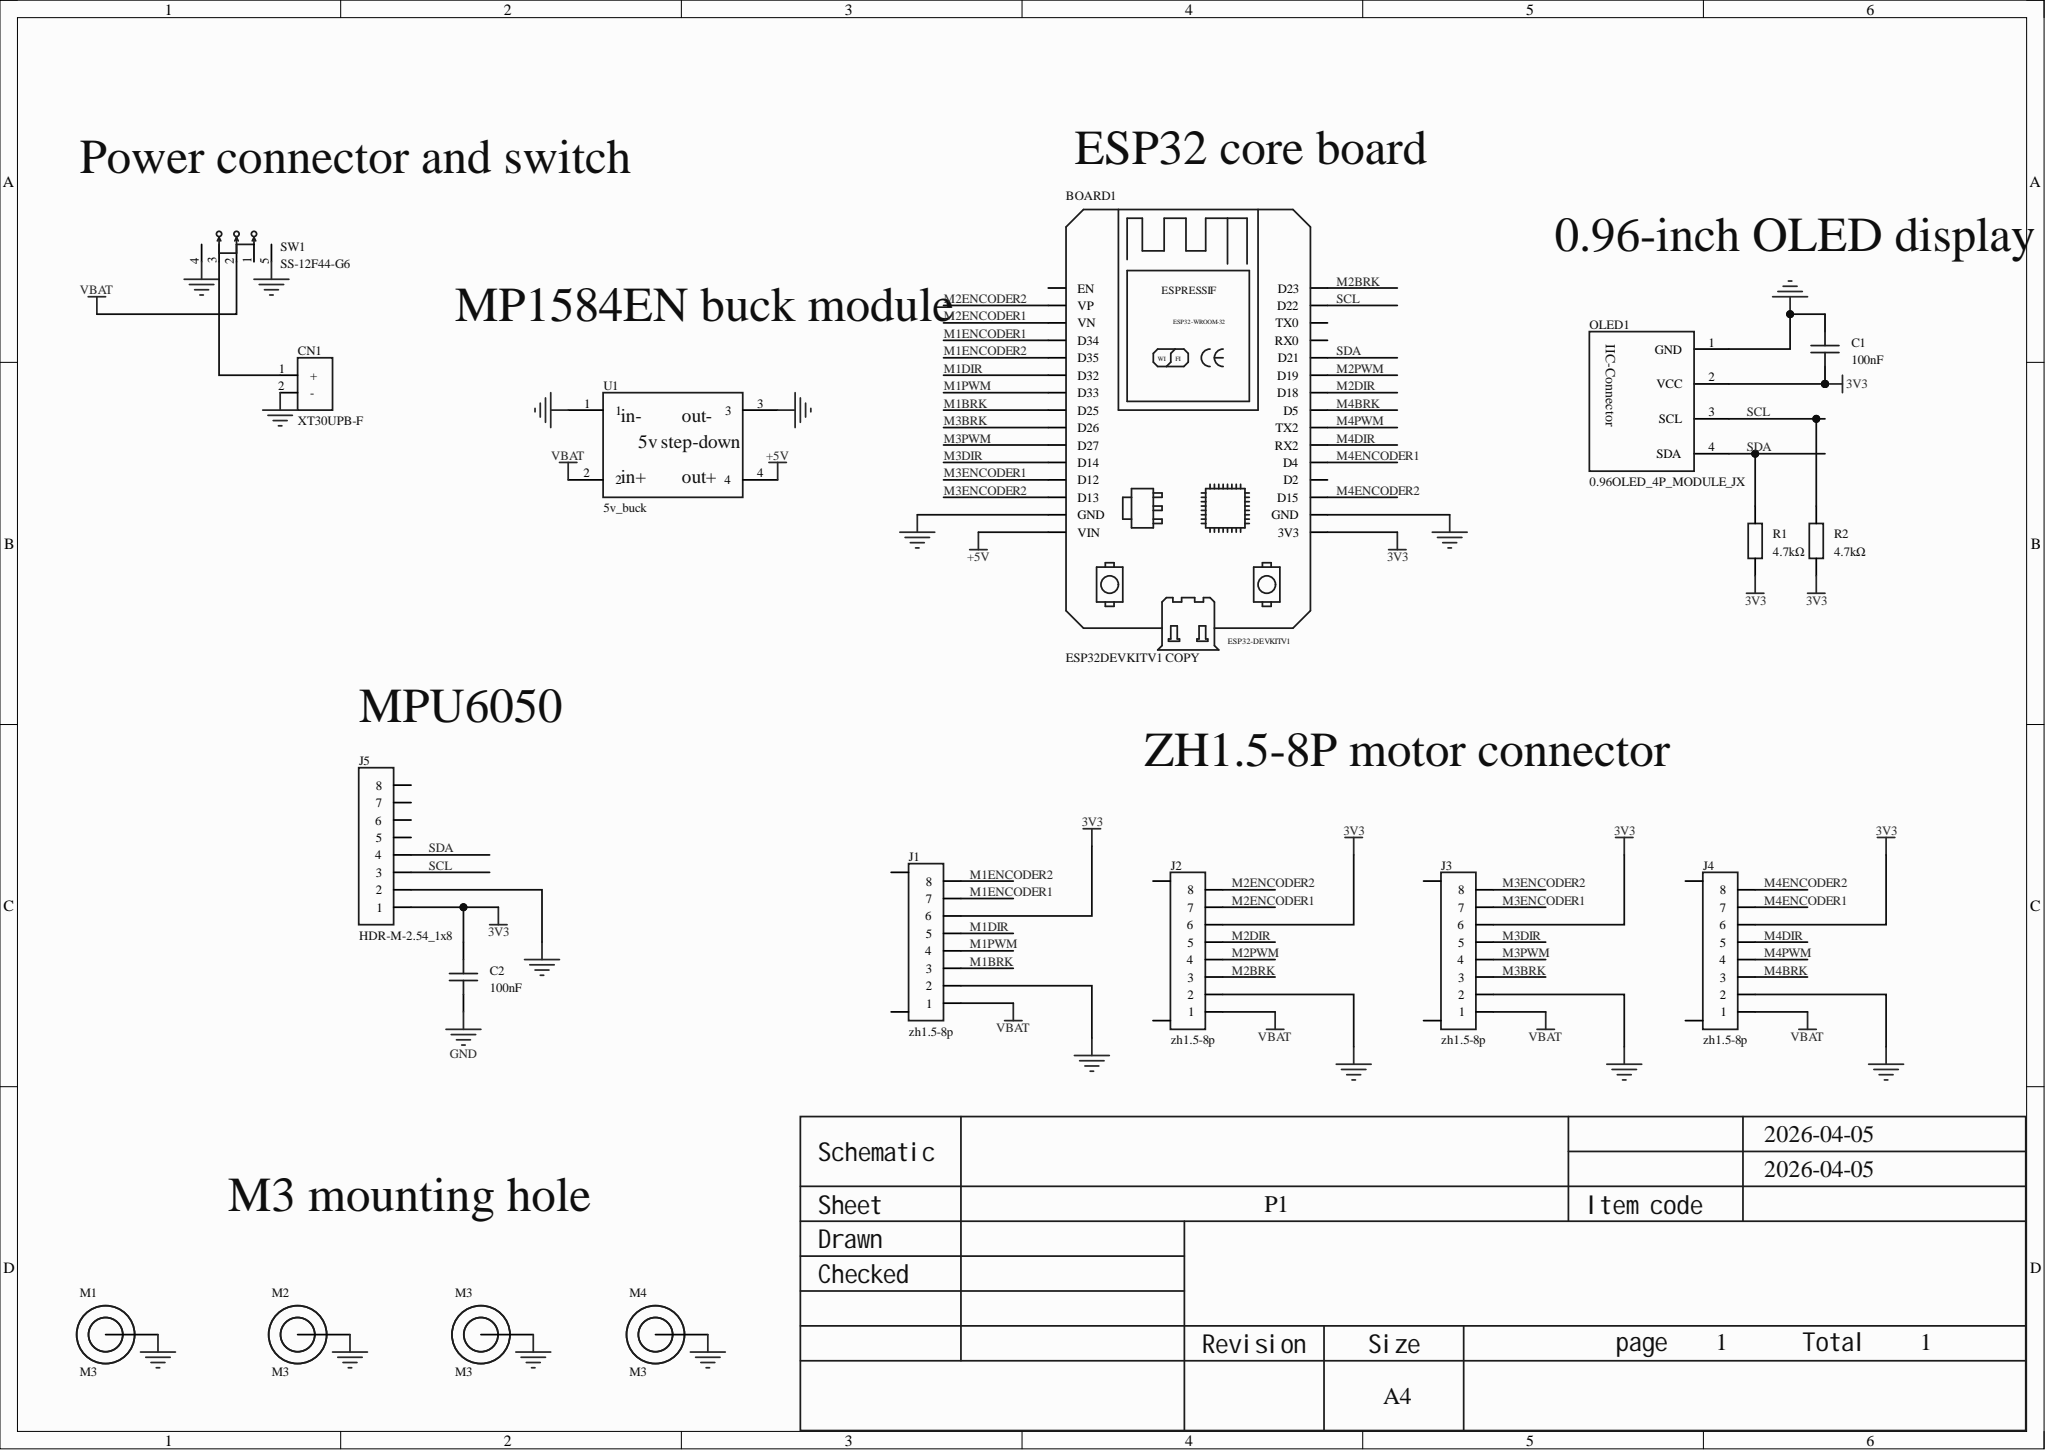Circuit board | Altium Designer | 18 parts | 27 nets
Bill of materials:
Comment,Description,Designator,Footprint,LibRef,Quantity
"ESP32DEVKITV1 COPY","","BOARD1","ESP32-DEVKITV1","ESP32DEVKITV1 COPY","1"
"100nF","","C1, C2","C0603","CAP_0603","2"
"XT30UPB-F","","CN1","XT30","XT30","1"
"zh1.5-8p","","J1, J2, J3, J4","ZH1.5-8P","zh1.5-8p","4"
"HDR-M-2.54_1x8","","J5","HDR-M-2.54_1X8","HDR-M-2.54_1x8","1"
"M3","","M1, M2, M3, M4","M3","M3","4"
"0.96OLED_4P_MODULE_JX","","OLED1","0.96OLED_4P","0.96OLED_4P_MODULE_JX","1"
"4.7kΩ","","R1, R2","Res_1/8W","Res_AXIAL-1/8W","2"
"SS-12F44-G6","","SW1","SW-TH_SS-12F44-GX","SS-12F44-G6","1"
"5v_buck","","U1","5V_BUCK","5v_buck","1"
Netlist (Protel format):
[
BOARD1
ESP32-DEVKITV1
ESP32DEVKITV1 COPY



]
[
C1
C0603
100nF



]
[
C2
C0603
100nF



]
[
CN1
XT30
XT30UPB-F



]
[
J1
ZH1.5-8P
zh1.5-8p



]
[
J2
ZH1.5-8P
zh1.5-8p



]
[
J3
ZH1.5-8P
zh1.5-8p



]
[
J4
ZH1.5-8P
zh1.5-8p



]
[
J5
HDR-M-2.54_1X8
HDR-M-2.54_1x8



]
[
M1
M3
M3



]
[
M2
M3
M3



]
[
M3
M3
M3



]
[
M4
M3
M3



]
[
OLED1
0.96OLED_4P
0.96OLED_4P_MODULE_JX



]
[
R1
Res_1/8W
4.7kΩ



]
[
R2
Res_1/8W
4.7kΩ



]
[
SW1
SW-TH_SS-12F44-GX
SS-12F44-G6



]
[
U1
5V_BUCK
5v_buck



]
(
VBAT
J1-1
J2-1
J3-1
J4-1
SW1-2
U1-2
)
(
SDA
BOARD1-D21
J5-4
OLED1-4
R1-2
)
(
SCL
BOARD1-D22
J5-3
OLED1-3
R2-2
)
(
NetCN1_1
CN1-1
SW1-3
)
(
M4PWM
BOARD1-TX2
J4-4
)
(
M4ENCODER2
BOARD1-D15
J4-8
)
(
M4ENCODER1
BOARD1-D4
J4-7
)
(
M4DIR
BOARD1-RX2
J4-5
)
(
M4BRK
BOARD1-D5
J4-3
)
(
M3PWM
BOARD1-D27
J3-4
)
(
M3ENCODER2
BOARD1-D13
J3-8
)
(
M3ENCODER1
BOARD1-D12
J3-7
)
(
M3DIR
BOARD1-D14
J3-5
)
(
M3BRK
BOARD1-D26
J3-3
)
(
M2PWM
BOARD1-D19
J2-4
)
(
M2ENCODER2
BOARD1-VP
J2-8
)
(
M2ENCODER1
BOARD1-VN
J2-7
)
(
M2DIR
BOARD1-D18
J2-5
)
(
M2BRK
BOARD1-D23
J2-3
)
(
M1PWM
BOARD1-D33
J1-4
)
(
M1ENCODER2
BOARD1-D35
J1-8
)
(
M1ENCODER1
BOARD1-D34
J1-7
)
(
M1DIR
BOARD1-D32
J1-5
)
(
M1BRK
BOARD1-D25
J1-3
)
(
GND
BOARD1-GND
BOARD1-GND@1
C1-2
C2-1
CN1-2
J1-2
J2-2
J3-2
J4-2
J5-2
M1-1
M2-1
M3-1
M4-1
OLED1-1
SW1-4
SW1-5
U1-1
U1-3
)
(
+5V
BOARD1-VIN
U1-4
)
(
3V3
BOARD1-3V3
C1-1
C2-2
J1-6
J2-6
J3-6
J4-6
J5-1
OLED1-2
R1-1
R2-1
)